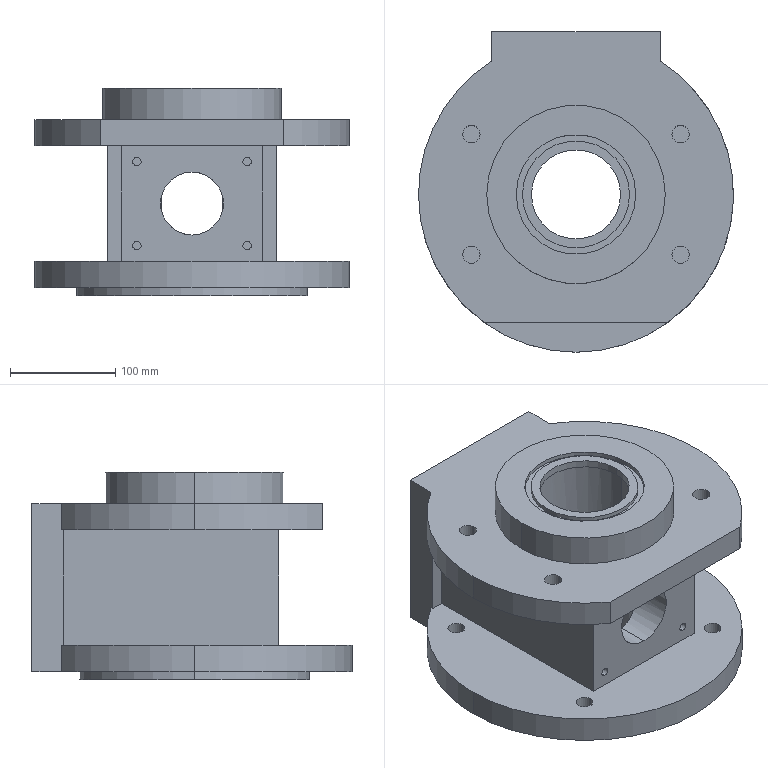Part | SolidWorks | features HoleWzd 8, ICE 6, Revolution 2, Extrusion 1 | 1 solid | 85 faces | box 300 x 305 x 198 mm | volume 5533662 mm3 | cylinder 55 | plane 30 | commonest cylinder face diameters 8 x8 10 x8 16 x8 16.5 x8 300 x6 99 x3